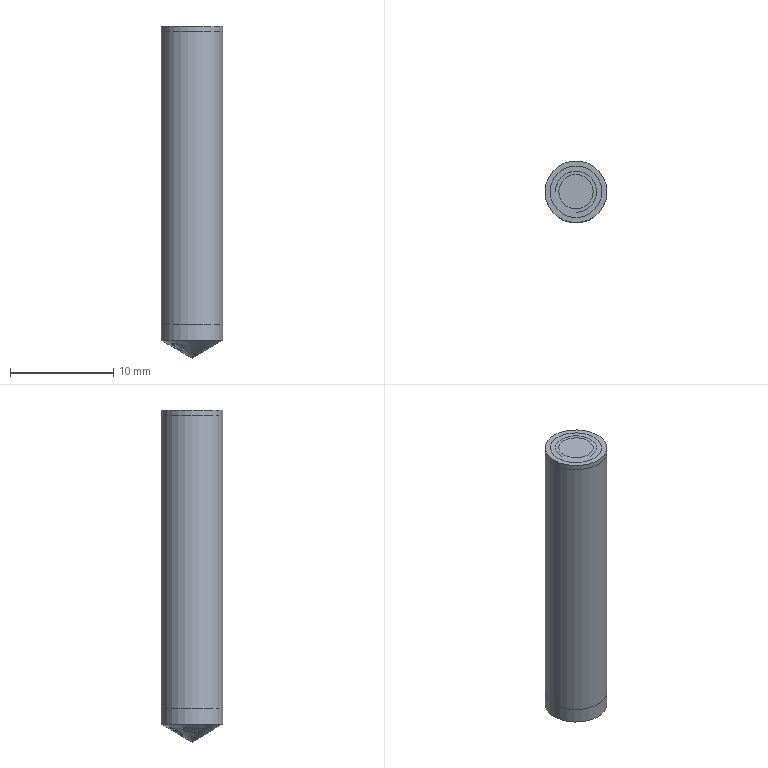Part | STEP file | E030603000 | 2 solids | 45 faces | box 6 x 6 x 32.232 mm | volume 1637 mm3 | plane 15 | other 13 | cone 11 | cylinder 5 | torus 1 | commonest cylinder face diameters 6 x2 3.333 x1 3.987 x1 4 x1